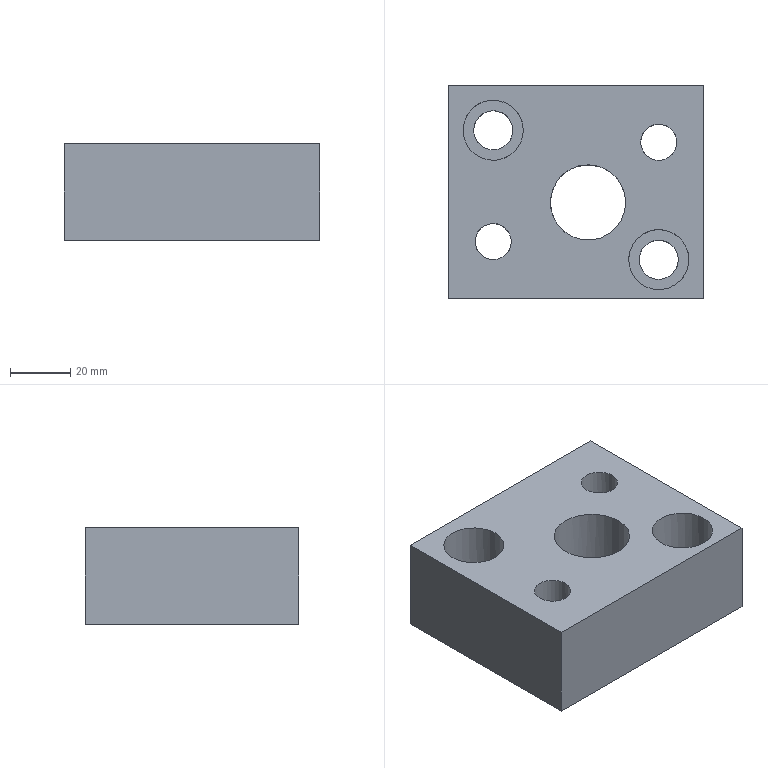Part | STEP file | gslz 2016.10.28-13_id1606_x_t | 1 solid | 17 faces | box 85 x 71 x 32 mm | volume 153487 mm3 | plane 9 | cylinder 8 | commonest cylinder face diameters 12 x2 13 x2 20 x2 25 x1 32 x1
STEP:
#1=CARTESIAN_POINT('',(0.,0.,0.));
#2=DIRECTION('',(0.,0.,1.));
#3=DIRECTION('',(1.,0.,0.));
#4=AXIS2_PLACEMENT_3D('',#1,#2,#3);
#5=CARTESIAN_POINT('',(-1393.372,235.,-32.));
#6=VERTEX_POINT('',#5);
#7=CARTESIAN_POINT('',(-1400.963,228.592,-32.));
#8=VERTEX_POINT('',#7);
#9=CARTESIAN_POINT('',(-1399.872,235.,-32.));
#10=DIRECTION('',(0.,0.,-1.));
#11=DIRECTION('',(1.,0.,0.));
#12=AXIS2_PLACEMENT_3D('',#9,#10,#11);
#13=CIRCLE('',#12,6.5);
#14=CARTESIAN_POINT('',(-1345.502,255.485,-32.));
#15=DIRECTION('',(0.,0.,1.));
#16=DIRECTION('',(1.,0.,0.));
#17=AXIS2_PLACEMENT_3D('',#14,#15,#16);
#18=PLANE('',#17);
#19=CARTESIAN_POINT('',(-47.871,-20.485));
#20=CARTESIAN_POINT('',(-47.871,-31.743));
#21=CARTESIAN_POINT('',(-57.621,-26.114));
#22=CARTESIAN_POINT('',(-67.371,-20.485));
#23=CARTESIAN_POINT('',(-57.621,-14.856));
#24=CARTESIAN_POINT('',(-47.871,-9.227));
#25=CARTESIAN_POINT('',(-47.871,-20.485));
#26=(BOUNDED_CURVE()B_SPLINE_CURVE(2,(#19,#20,#21,#22,#23,#24,#25),.UNSPECIFIED.,.T.,.F.)B_SPLINE_CURVE_WITH_KNOTS((1,2,2,2,2,1),(-2.094,0.,2.094,4.189,6.283,8.378),.UNSPECIFIED.)CURVE()GEOMETRIC_REPRESENTATION_ITEM()RATIONAL_B_SPLINE_CURVE((1.,0.5,1.,0.5,1.,0.5,1.))REPRESENTATION_ITEM(''));
#27=(GEOMETRIC_REPRESENTATION_CONTEXT(2)PARAMETRIC_REPRESENTATION_CONTEXT()REPRESENTATION_CONTEXT('',''));
#28=DEFINITIONAL_REPRESENTATION('',(#26),#27);
#29=PCURVE('',#18,#28);
#30=CARTESIAN_POINT('',(-1399.872,235.,-0.5408));
#31=DIRECTION('',(0.,0.,-1.));
#32=DIRECTION('',(-1.,0.,0.));
#33=AXIS2_PLACEMENT_3D('',#30,#31,#32);
#34=CYLINDRICAL_SURFACE('',#33,6.5);
#35=CARTESIAN_POINT('',(9.425,31.459));
#36=DIRECTION('',(1.,0.));
#37=VECTOR('',#36,1.);
#38=LINE('',#35,#37);
#39=(GEOMETRIC_REPRESENTATION_CONTEXT(2)PARAMETRIC_REPRESENTATION_CONTEXT()REPRESENTATION_CONTEXT('',''));
#40=DEFINITIONAL_REPRESENTATION('',(#38),#39);
#41=PCURVE('',#34,#40);
#42=SURFACE_CURVE('',#13,(#29,#41),.PCURVE_S1.);
#43=EDGE_CURVE('',#6,#8,#42,.T.);
#44=ORIENTED_EDGE('',*,*,#43,.F.);
#45=CARTESIAN_POINT('',(-1399.872,235.,-32.));
#46=DIRECTION('',(0.,0.,-1.));
#47=DIRECTION('',(1.,0.,0.));
#48=AXIS2_PLACEMENT_3D('',#45,#46,#47);
#49=CIRCLE('',#48,6.5);
#50=CARTESIAN_POINT('',(-47.871,-20.485));
#51=CARTESIAN_POINT('',(-47.871,-31.743));
#52=CARTESIAN_POINT('',(-57.621,-26.114));
#53=CARTESIAN_POINT('',(-67.371,-20.485));
#54=CARTESIAN_POINT('',(-57.621,-14.856));
#55=CARTESIAN_POINT('',(-47.871,-9.227));
#56=CARTESIAN_POINT('',(-47.871,-20.485));
#57=(BOUNDED_CURVE()B_SPLINE_CURVE(2,(#50,#51,#52,#53,#54,#55,#56),.UNSPECIFIED.,.T.,.F.)B_SPLINE_CURVE_WITH_KNOTS((1,2,2,2,2,1),(-2.094,0.,2.094,4.189,6.283,8.378),.UNSPECIFIED.)CURVE()GEOMETRIC_REPRESENTATION_ITEM()RATIONAL_B_SPLINE_CURVE((1.,0.5,1.,0.5,1.,0.5,1.))REPRESENTATION_ITEM(''));
#58=(GEOMETRIC_REPRESENTATION_CONTEXT(2)PARAMETRIC_REPRESENTATION_CONTEXT()REPRESENTATION_CONTEXT('',''));
#59=DEFINITIONAL_REPRESENTATION('',(#57),#58);
#60=PCURVE('',#18,#59);
#61=CARTESIAN_POINT('',(3.142,31.459));
#62=DIRECTION('',(1.,0.));
#63=VECTOR('',#62,1.);
#64=LINE('',#61,#63);
#65=(GEOMETRIC_REPRESENTATION_CONTEXT(2)PARAMETRIC_REPRESENTATION_CONTEXT()REPRESENTATION_CONTEXT('',''));
#66=DEFINITIONAL_REPRESENTATION('',(#64),#65);
#67=PCURVE('',#34,#66);
#68=SURFACE_CURVE('',#49,(#60,#67),.PCURVE_S1.);
#69=EDGE_CURVE('',#8,#6,#68,.T.);
#70=ORIENTED_EDGE('',*,*,#69,.F.);
#71=EDGE_LOOP('',(#44,#70));
#72=FACE_BOUND('',#71,.T.);
#73=CARTESIAN_POINT('',(-1453.551,246.853,-32.));
#74=VERTEX_POINT('',#73);
#75=CARTESIAN_POINT('',(-1454.872,241.,-32.));
#76=DIRECTION('',(0.,0.,1.));
#77=DIRECTION('',(0.2202,0.9754,0.));
#78=AXIS2_PLACEMENT_3D('',#75,#76,#77);
#79=CIRCLE('',#78,6.);
#80=CARTESIAN_POINT('',(-109.371,-14.485));
#81=DIRECTION('',(0.2202,0.9754));
#82=AXIS2_PLACEMENT_2D('',#80,#81);
#83=CIRCLE('',#82,6.);
#84=(GEOMETRIC_REPRESENTATION_CONTEXT(2)PARAMETRIC_REPRESENTATION_CONTEXT()REPRESENTATION_CONTEXT('',''));
#85=DEFINITIONAL_REPRESENTATION('',(#83),#84);
#86=PCURVE('',#18,#85);
#87=CARTESIAN_POINT('',(-1454.872,241.,-9.));
#88=DIRECTION('',(0.,0.,-1.));
#89=DIRECTION('',(-1.,0.,0.));
#90=AXIS2_PLACEMENT_3D('',#87,#88,#89);
#91=CYLINDRICAL_SURFACE('',#90,6.);
#92=CARTESIAN_POINT('',(8.076,23.));
#93=DIRECTION('',(-1.,0.));
#94=VECTOR('',#93,1.);
#95=LINE('',#92,#94);
#96=(GEOMETRIC_REPRESENTATION_CONTEXT(2)PARAMETRIC_REPRESENTATION_CONTEXT()REPRESENTATION_CONTEXT('',''));
#97=DEFINITIONAL_REPRESENTATION('',(#95),#96);
#98=PCURVE('',#91,#97);
#99=SURFACE_CURVE('',#79,(#86,#98),.PCURVE_S1.);
#100=EDGE_CURVE('',#74,#74,#99,.T.);
#101=ORIENTED_EDGE('',*,*,#100,.T.);
#102=EDGE_LOOP('',(#101));
#103=FACE_BOUND('',#102,.T.);
#104=CARTESIAN_POINT('',(-1448.372,278.,-32.));
#105=VERTEX_POINT('',#104);
#106=CARTESIAN_POINT('',(-1455.963,271.592,-32.));
#107=VERTEX_POINT('',#106);
#108=CARTESIAN_POINT('',(-1454.872,278.,-32.));
#109=DIRECTION('',(0.,0.,-1.));
#110=DIRECTION('',(1.,0.,0.));
#111=AXIS2_PLACEMENT_3D('',#108,#109,#110);
#112=CIRCLE('',#111,6.5);
#113=CARTESIAN_POINT('',(-102.871,22.515));
#114=CARTESIAN_POINT('',(-102.871,11.257));
#115=CARTESIAN_POINT('',(-112.621,16.886));
#116=CARTESIAN_POINT('',(-122.371,22.515));
#117=CARTESIAN_POINT('',(-112.621,28.144));
#118=CARTESIAN_POINT('',(-102.871,33.773));
#119=CARTESIAN_POINT('',(-102.871,22.515));
#120=(BOUNDED_CURVE()B_SPLINE_CURVE(2,(#113,#114,#115,#116,#117,#118,#119),.UNSPECIFIED.,.T.,.F.)B_SPLINE_CURVE_WITH_KNOTS((1,2,2,2,2,1),(-2.094,0.,2.094,4.189,6.283,8.378),.UNSPECIFIED.)CURVE()GEOMETRIC_REPRESENTATION_ITEM()RATIONAL_B_SPLINE_CURVE((1.,0.5,1.,0.5,1.,0.5,1.))REPRESENTATION_ITEM(''));
#121=(GEOMETRIC_REPRESENTATION_CONTEXT(2)PARAMETRIC_REPRESENTATION_CONTEXT()REPRESENTATION_CONTEXT('',''));
#122=DEFINITIONAL_REPRESENTATION('',(#120),#121);
#123=PCURVE('',#18,#122);
#124=CARTESIAN_POINT('',(-1454.872,278.,-0.5408));
#125=DIRECTION('',(0.,0.,-1.));
#126=DIRECTION('',(-1.,0.,0.));
#127=AXIS2_PLACEMENT_3D('',#124,#125,#126);
#128=CYLINDRICAL_SURFACE('',#127,6.5);
#129=CARTESIAN_POINT('',(9.425,31.459));
#130=DIRECTION('',(1.,0.));
#131=VECTOR('',#130,1.);
#132=LINE('',#129,#131);
#133=(GEOMETRIC_REPRESENTATION_CONTEXT(2)PARAMETRIC_REPRESENTATION_CONTEXT()REPRESENTATION_CONTEXT('',''));
#134=DEFINITIONAL_REPRESENTATION('',(#132),#133);
#135=PCURVE('',#128,#134);
#136=SURFACE_CURVE('',#112,(#123,#135),.PCURVE_S1.);
#137=EDGE_CURVE('',#105,#107,#136,.T.);
#138=ORIENTED_EDGE('',*,*,#137,.F.);
#139=CARTESIAN_POINT('',(-1454.872,278.,-32.));
#140=DIRECTION('',(0.,0.,-1.));
#141=DIRECTION('',(1.,0.,0.));
#142=AXIS2_PLACEMENT_3D('',#139,#140,#141);
#143=CIRCLE('',#142,6.5);
#144=CARTESIAN_POINT('',(-102.871,22.515));
#145=CARTESIAN_POINT('',(-102.871,11.257));
#146=CARTESIAN_POINT('',(-112.621,16.886));
#147=CARTESIAN_POINT('',(-122.371,22.515));
#148=CARTESIAN_POINT('',(-112.621,28.144));
#149=CARTESIAN_POINT('',(-102.871,33.773));
#150=CARTESIAN_POINT('',(-102.871,22.515));
#151=(BOUNDED_CURVE()B_SPLINE_CURVE(2,(#144,#145,#146,#147,#148,#149,#150),.UNSPECIFIED.,.T.,.F.)B_SPLINE_CURVE_WITH_KNOTS((1,2,2,2,2,1),(-2.094,0.,2.094,4.189,6.283,8.378),.UNSPECIFIED.)CURVE()GEOMETRIC_REPRESENTATION_ITEM()RATIONAL_B_SPLINE_CURVE((1.,0.5,1.,0.5,1.,0.5,1.))REPRESENTATION_ITEM(''));
#152=(GEOMETRIC_REPRESENTATION_CONTEXT(2)PARAMETRIC_REPRESENTATION_CONTEXT()REPRESENTATION_CONTEXT('',''));
#153=DEFINITIONAL_REPRESENTATION('',(#151),#152);
#154=PCURVE('',#18,#153);
#155=CARTESIAN_POINT('',(3.142,31.459));
#156=DIRECTION('',(1.,0.));
#157=VECTOR('',#156,1.);
#158=LINE('',#155,#157);
#159=(GEOMETRIC_REPRESENTATION_CONTEXT(2)PARAMETRIC_REPRESENTATION_CONTEXT()REPRESENTATION_CONTEXT('',''));
#160=DEFINITIONAL_REPRESENTATION('',(#158),#159);
#161=PCURVE('',#128,#160);
#162=SURFACE_CURVE('',#143,(#154,#161),.PCURVE_S1.);
#163=EDGE_CURVE('',#107,#105,#162,.T.);
#164=ORIENTED_EDGE('',*,*,#163,.F.);
#165=EDGE_LOOP('',(#138,#164));
#166=FACE_BOUND('',#165,.T.);
#167=CARTESIAN_POINT('',(-1384.872,293.,-32.));
#168=VERTEX_POINT('',#167);
#169=CARTESIAN_POINT('',(-1469.872,293.,-32.));
#170=VERTEX_POINT('',#169);
#171=CARTESIAN_POINT('',(-1423.372,293.,-32.));
#172=DIRECTION('',(-1.,0.,0.));
#173=VECTOR('',#172,1.);
#174=LINE('',#171,#173);
#175=CARTESIAN_POINT('',(-77.871,37.515));
#176=DIRECTION('',(-1.,0.));
#177=VECTOR('',#176,1.);
#178=LINE('',#175,#177);
#179=(GEOMETRIC_REPRESENTATION_CONTEXT(2)PARAMETRIC_REPRESENTATION_CONTEXT()REPRESENTATION_CONTEXT('',''));
#180=DEFINITIONAL_REPRESENTATION('',(#178),#179);
#181=PCURVE('',#18,#180);
#182=CARTESIAN_POINT('',(-1423.372,293.,-56.));
#183=DIRECTION('',(0.,1.,0.));
#184=DIRECTION('',(0.,0.,1.));
#185=AXIS2_PLACEMENT_3D('',#182,#183,#184);
#186=PLANE('',#185);
#187=CARTESIAN_POINT('',(24.,0.));
#188=DIRECTION('',(0.,-1.));
#189=VECTOR('',#188,1.);
#190=LINE('',#187,#189);
#191=(GEOMETRIC_REPRESENTATION_CONTEXT(2)PARAMETRIC_REPRESENTATION_CONTEXT()REPRESENTATION_CONTEXT('',''));
#192=DEFINITIONAL_REPRESENTATION('',(#190),#191);
#193=PCURVE('',#186,#192);
#194=SURFACE_CURVE('',#174,(#181,#193),.PCURVE_S1.);
#195=EDGE_CURVE('',#168,#170,#194,.T.);
#196=ORIENTED_EDGE('',*,*,#195,.F.);
#197=CARTESIAN_POINT('',(-1384.872,222.,-32.));
#198=VERTEX_POINT('',#197);
#199=CARTESIAN_POINT('',(-1384.872,336.,-32.));
#200=DIRECTION('',(0.,1.,0.));
#201=VECTOR('',#200,1.);
#202=LINE('',#199,#201);
#203=CARTESIAN_POINT('',(-39.371,80.515));
#204=DIRECTION('',(0.,1.));
#205=VECTOR('',#204,1.);
#206=LINE('',#203,#205);
#207=(GEOMETRIC_REPRESENTATION_CONTEXT(2)PARAMETRIC_REPRESENTATION_CONTEXT()REPRESENTATION_CONTEXT('',''));
#208=DEFINITIONAL_REPRESENTATION('',(#206),#207);
#209=PCURVE('',#18,#208);
#210=CARTESIAN_POINT('',(-1384.872,336.,-56.));
#211=DIRECTION('',(1.,0.,0.));
#212=DIRECTION('',(0.,0.,-1.));
#213=AXIS2_PLACEMENT_3D('',#210,#211,#212);
#214=PLANE('',#213);
#215=CARTESIAN_POINT('',(-24.,0.));
#216=DIRECTION('',(0.,1.));
#217=VECTOR('',#216,1.);
#218=LINE('',#215,#217);
#219=(GEOMETRIC_REPRESENTATION_CONTEXT(2)PARAMETRIC_REPRESENTATION_CONTEXT()REPRESENTATION_CONTEXT('',''));
#220=DEFINITIONAL_REPRESENTATION('',(#218),#219);
#221=PCURVE('',#214,#220);
#222=SURFACE_CURVE('',#202,(#209,#221),.PCURVE_S1.);
#223=EDGE_CURVE('',#198,#168,#222,.T.);
#224=ORIENTED_EDGE('',*,*,#223,.F.);
#225=CARTESIAN_POINT('',(-1469.872,222.,-32.));
#226=VERTEX_POINT('',#225);
#227=CARTESIAN_POINT('',(-1423.372,222.,-32.));
#228=DIRECTION('',(1.,0.,0.));
#229=VECTOR('',#228,1.);
#230=LINE('',#227,#229);
#231=CARTESIAN_POINT('',(-77.871,-33.485));
#232=DIRECTION('',(1.,0.));
#233=VECTOR('',#232,1.);
#234=LINE('',#231,#233);
#235=(GEOMETRIC_REPRESENTATION_CONTEXT(2)PARAMETRIC_REPRESENTATION_CONTEXT()REPRESENTATION_CONTEXT('',''));
#236=DEFINITIONAL_REPRESENTATION('',(#234),#235);
#237=PCURVE('',#18,#236);
#238=CARTESIAN_POINT('',(-1423.372,222.,-56.));
#239=DIRECTION('',(0.,-1.,0.));
#240=DIRECTION('',(0.,0.,-1.));
#241=AXIS2_PLACEMENT_3D('',#238,#239,#240);
#242=PLANE('',#241);
#243=CARTESIAN_POINT('',(-24.,0.));
#244=DIRECTION('',(0.,1.));
#245=VECTOR('',#244,1.);
#246=LINE('',#243,#245);
#247=(GEOMETRIC_REPRESENTATION_CONTEXT(2)PARAMETRIC_REPRESENTATION_CONTEXT()REPRESENTATION_CONTEXT('',''));
#248=DEFINITIONAL_REPRESENTATION('',(#246),#247);
#249=PCURVE('',#242,#248);
#250=SURFACE_CURVE('',#230,(#237,#249),.PCURVE_S1.);
#251=EDGE_CURVE('',#226,#198,#250,.T.);
#252=ORIENTED_EDGE('',*,*,#251,.F.);
#253=CARTESIAN_POINT('',(-1469.872,336.,-32.));
#254=DIRECTION('',(0.,-1.,0.));
#255=VECTOR('',#254,1.);
#256=LINE('',#253,#255);
#257=CARTESIAN_POINT('',(-124.371,80.515));
#258=DIRECTION('',(0.,-1.));
#259=VECTOR('',#258,1.);
#260=LINE('',#257,#259);
#261=(GEOMETRIC_REPRESENTATION_CONTEXT(2)PARAMETRIC_REPRESENTATION_CONTEXT()REPRESENTATION_CONTEXT('',''));
#262=DEFINITIONAL_REPRESENTATION('',(#260),#261);
#263=PCURVE('',#18,#262);
#264=CARTESIAN_POINT('',(-1469.872,336.,-56.));
#265=DIRECTION('',(-1.,0.,0.));
#266=DIRECTION('',(0.,0.,1.));
#267=AXIS2_PLACEMENT_3D('',#264,#265,#266);
#268=PLANE('',#267);
#269=CARTESIAN_POINT('',(24.,0.));
#270=DIRECTION('',(0.,-1.));
#271=VECTOR('',#270,1.);
#272=LINE('',#269,#271);
#273=(GEOMETRIC_REPRESENTATION_CONTEXT(2)PARAMETRIC_REPRESENTATION_CONTEXT()REPRESENTATION_CONTEXT('',''));
#274=DEFINITIONAL_REPRESENTATION('',(#272),#273);
#275=PCURVE('',#268,#274);
#276=SURFACE_CURVE('',#256,(#263,#275),.PCURVE_S1.);
#277=EDGE_CURVE('',#170,#226,#276,.T.);
#278=ORIENTED_EDGE('',*,*,#277,.F.);
#279=EDGE_LOOP('',(#196,#224,#252,#278));
#280=FACE_BOUND('',#279,.T.);
#281=CARTESIAN_POINT('',(-1407.372,254.,-32.));
#282=VERTEX_POINT('',#281);
#283=CARTESIAN_POINT('',(-1423.372,254.,-32.));
#284=DIRECTION('',(0.,0.,-1.));
#285=DIRECTION('',(1.,0.,0.));
#286=AXIS2_PLACEMENT_3D('',#283,#284,#285);
#287=CIRCLE('',#286,16.);
#288=CARTESIAN_POINT('',(-61.871,-1.485));
#289=CARTESIAN_POINT('',(-61.871,-29.198));
#290=CARTESIAN_POINT('',(-85.871,-15.341));
#291=CARTESIAN_POINT('',(-109.871,-1.485));
#292=CARTESIAN_POINT('',(-85.871,12.372));
#293=CARTESIAN_POINT('',(-61.871,26.228));
#294=CARTESIAN_POINT('',(-61.871,-1.485));
#295=(BOUNDED_CURVE()B_SPLINE_CURVE(2,(#288,#289,#290,#291,#292,#293,#294),.UNSPECIFIED.,.T.,.F.)B_SPLINE_CURVE_WITH_KNOTS((1,2,2,2,2,1),(-2.094,0.,2.094,4.189,6.283,8.378),.UNSPECIFIED.)CURVE()GEOMETRIC_REPRESENTATION_ITEM()RATIONAL_B_SPLINE_CURVE((1.,0.5,1.,0.5,1.,0.5,1.))REPRESENTATION_ITEM(''));
#296=(GEOMETRIC_REPRESENTATION_CONTEXT(2)PARAMETRIC_REPRESENTATION_CONTEXT()REPRESENTATION_CONTEXT('',''));
#297=DEFINITIONAL_REPRESENTATION('',(#295),#296);
#298=PCURVE('',#18,#297);
#299=CARTESIAN_POINT('',(-1423.372,254.,-32.5));
#300=DIRECTION('',(0.,0.,1.));
#301=DIRECTION('',(0.,-1.,0.));
#302=AXIS2_PLACEMENT_3D('',#299,#300,#301);
#303=CYLINDRICAL_SURFACE('',#302,16.);
#304=CARTESIAN_POINT('',(7.854,0.5));
#305=DIRECTION('',(-1.,0.));
#306=VECTOR('',#305,1.);
#307=LINE('',#304,#306);
#308=(GEOMETRIC_REPRESENTATION_CONTEXT(2)PARAMETRIC_REPRESENTATION_CONTEXT()REPRESENTATION_CONTEXT('',''));
#309=DEFINITIONAL_REPRESENTATION('',(#307),#308);
#310=PCURVE('',#303,#309);
#311=SURFACE_CURVE('',#287,(#298,#310),.PCURVE_S1.);
#312=EDGE_CURVE('',#282,#282,#311,.T.);
#313=ORIENTED_EDGE('',*,*,#312,.F.);
#314=EDGE_LOOP('',(#313));
#315=FACE_BOUND('',#314,.T.);
#316=CARTESIAN_POINT('',(-1398.551,279.853,-32.));
#317=VERTEX_POINT('',#316);
#318=CARTESIAN_POINT('',(-1399.872,274.,-32.));
#319=DIRECTION('',(0.,0.,1.));
#320=DIRECTION('',(0.2202,0.9754,0.));
#321=AXIS2_PLACEMENT_3D('',#318,#319,#320);
#322=CIRCLE('',#321,6.);
#323=CARTESIAN_POINT('',(-54.371,18.515));
#324=DIRECTION('',(0.2202,0.9754));
#325=AXIS2_PLACEMENT_2D('',#323,#324);
#326=CIRCLE('',#325,6.);
#327=(GEOMETRIC_REPRESENTATION_CONTEXT(2)PARAMETRIC_REPRESENTATION_CONTEXT()REPRESENTATION_CONTEXT('',''));
#328=DEFINITIONAL_REPRESENTATION('',(#326),#327);
#329=PCURVE('',#18,#328);
#330=CARTESIAN_POINT('',(-1399.872,274.,-9.));
#331=DIRECTION('',(0.,0.,-1.));
#332=DIRECTION('',(-1.,0.,0.));
#333=AXIS2_PLACEMENT_3D('',#330,#331,#332);
#334=CYLINDRICAL_SURFACE('',#333,6.);
#335=CARTESIAN_POINT('',(8.076,23.));
#336=DIRECTION('',(-1.,0.));
#337=VECTOR('',#336,1.);
#338=LINE('',#335,#337);
#339=(GEOMETRIC_REPRESENTATION_CONTEXT(2)PARAMETRIC_REPRESENTATION_CONTEXT()REPRESENTATION_CONTEXT('',''));
#340=DEFINITIONAL_REPRESENTATION('',(#338),#339);
#341=PCURVE('',#334,#340);
#342=SURFACE_CURVE('',#322,(#329,#341),.PCURVE_S1.);
#343=EDGE_CURVE('',#317,#317,#342,.T.);
#344=ORIENTED_EDGE('',*,*,#343,.T.);
#345=EDGE_LOOP('',(#344));
#346=FACE_BOUND('',#345,.T.);
#347=ADVANCED_FACE('',(#72,#103,#166,#280,#315,#346),#18,.F.);
#348=CARTESIAN_POINT('',(-1389.872,235.,0.));
#349=VERTEX_POINT('',#348);
#350=CARTESIAN_POINT('',(-1401.551,225.142,0.));
#351=VERTEX_POINT('',#350);
#352=CARTESIAN_POINT('',(-1399.872,235.,0.));
#353=DIRECTION('',(0.,0.,1.));
#354=DIRECTION('',(1.,0.,0.));
#355=AXIS2_PLACEMENT_3D('',#352,#353,#354);
#356=CIRCLE('',#355,10.);
#357=CARTESIAN_POINT('',(-1423.372,336.,0.));
#358=DIRECTION('',(0.,0.,1.));
#359=DIRECTION('',(0.,-1.,0.));
#360=AXIS2_PLACEMENT_3D('',#357,#358,#359);
#361=PLANE('',#360);
#362=CARTESIAN_POINT('',(101.,23.5));
#363=DIRECTION('',(0.,1.));
#364=AXIS2_PLACEMENT_2D('',#362,#363);
#365=CIRCLE('',#364,10.);
#366=(GEOMETRIC_REPRESENTATION_CONTEXT(2)PARAMETRIC_REPRESENTATION_CONTEXT()REPRESENTATION_CONTEXT('',''));
#367=DEFINITIONAL_REPRESENTATION('',(#365),#366);
#368=PCURVE('',#361,#367);
#369=CARTESIAN_POINT('',(-1399.872,235.,-0.5408));
#370=DIRECTION('',(0.,0.,-1.));
#371=DIRECTION('',(-1.,0.,0.));
#372=AXIS2_PLACEMENT_3D('',#369,#370,#371);
#373=CYLINDRICAL_SURFACE('',#372,10.);
#374=CARTESIAN_POINT('',(9.425,-0.5408));
#375=DIRECTION('',(-1.,0.));
#376=VECTOR('',#375,1.);
#377=LINE('',#374,#376);
#378=(GEOMETRIC_REPRESENTATION_CONTEXT(2)PARAMETRIC_REPRESENTATION_CONTEXT()REPRESENTATION_CONTEXT('',''));
#379=DEFINITIONAL_REPRESENTATION('',(#377),#378);
#380=PCURVE('',#373,#379);
#381=SURFACE_CURVE('',#356,(#368,#380),.PCURVE_S1.);
#382=EDGE_CURVE('',#349,#351,#381,.T.);
#383=ORIENTED_EDGE('',*,*,#382,.F.);
#384=CARTESIAN_POINT('',(-1399.872,235.,0.));
#385=DIRECTION('',(0.,0.,1.));
#386=DIRECTION('',(1.,0.,0.));
#387=AXIS2_PLACEMENT_3D('',#384,#385,#386);
#388=CIRCLE('',#387,10.);
#389=CARTESIAN_POINT('',(101.,23.5));
#390=DIRECTION('',(0.,1.));
#391=AXIS2_PLACEMENT_2D('',#389,#390);
#392=CIRCLE('',#391,10.);
#393=(GEOMETRIC_REPRESENTATION_CONTEXT(2)PARAMETRIC_REPRESENTATION_CONTEXT()REPRESENTATION_CONTEXT('',''));
#394=DEFINITIONAL_REPRESENTATION('',(#392),#393);
#395=PCURVE('',#361,#394);
#396=CARTESIAN_POINT('',(15.708,-0.5408));
#397=DIRECTION('',(-1.,0.));
#398=VECTOR('',#397,1.);
#399=LINE('',#396,#398);
#400=(GEOMETRIC_REPRESENTATION_CONTEXT(2)PARAMETRIC_REPRESENTATION_CONTEXT()REPRESENTATION_CONTEXT('',''));
#401=DEFINITIONAL_REPRESENTATION('',(#399),#400);
#402=PCURVE('',#373,#401);
#403=SURFACE_CURVE('',#388,(#395,#402),.PCURVE_S1.);
#404=EDGE_CURVE('',#351,#349,#403,.T.);
#405=ORIENTED_EDGE('',*,*,#404,.F.);
#406=EDGE_LOOP('',(#383,#405));
#407=FACE_BOUND('',#406,.T.);
#408=CARTESIAN_POINT('',(-1393.872,274.,0.));
#409=VERTEX_POINT('',#408);
#410=CARTESIAN_POINT('',(-1398.551,279.853,0.));
#411=VERTEX_POINT('',#410);
#412=CARTESIAN_POINT('',(-1399.872,274.,0.));
#413=DIRECTION('',(0.,0.,1.));
#414=DIRECTION('',(1.,0.,0.));
#415=AXIS2_PLACEMENT_3D('',#412,#413,#414);
#416=CIRCLE('',#415,6.);
#417=CARTESIAN_POINT('',(62.,23.5));
#418=DIRECTION('',(0.,1.));
#419=AXIS2_PLACEMENT_2D('',#417,#418);
#420=CIRCLE('',#419,6.);
#421=(GEOMETRIC_REPRESENTATION_CONTEXT(2)PARAMETRIC_REPRESENTATION_CONTEXT()REPRESENTATION_CONTEXT('',''));
#422=DEFINITIONAL_REPRESENTATION('',(#420),#421);
#423=PCURVE('',#361,#422);
#424=CARTESIAN_POINT('',(3.142,-9.));
#425=DIRECTION('',(-1.,0.));
#426=VECTOR('',#425,1.);
#427=LINE('',#424,#426);
#428=(GEOMETRIC_REPRESENTATION_CONTEXT(2)PARAMETRIC_REPRESENTATION_CONTEXT()REPRESENTATION_CONTEXT('',''));
#429=DEFINITIONAL_REPRESENTATION('',(#427),#428);
#430=PCURVE('',#334,#429);
#431=SURFACE_CURVE('',#416,(#423,#430),.PCURVE_S1.);
#432=EDGE_CURVE('',#409,#411,#431,.T.);
#433=ORIENTED_EDGE('',*,*,#432,.F.);
#434=CARTESIAN_POINT('',(-1399.872,274.,0.));
#435=DIRECTION('',(0.,0.,1.));
#436=DIRECTION('',(1.,0.,0.));
#437=AXIS2_PLACEMENT_3D('',#434,#435,#436);
#438=CIRCLE('',#437,6.);
#439=CARTESIAN_POINT('',(62.,23.5));
#440=DIRECTION('',(0.,1.));
#441=AXIS2_PLACEMENT_2D('',#439,#440);
#442=CIRCLE('',#441,6.);
#443=(GEOMETRIC_REPRESENTATION_CONTEXT(2)PARAMETRIC_REPRESENTATION_CONTEXT()REPRESENTATION_CONTEXT('',''));
#444=DEFINITIONAL_REPRESENTATION('',(#442),#443);
#445=PCURVE('',#361,#444);
#446=CARTESIAN_POINT('',(9.425,-9.));
#447=DIRECTION('',(-1.,0.));
#448=VECTOR('',#447,1.);
#449=LINE('',#446,#448);
#450=(GEOMETRIC_REPRESENTATION_CONTEXT(2)PARAMETRIC_REPRESENTATION_CONTEXT()REPRESENTATION_CONTEXT('',''));
#451=DEFINITIONAL_REPRESENTATION('',(#449),#450);
#452=PCURVE('',#334,#451);
#453=SURFACE_CURVE('',#438,(#445,#452),.PCURVE_S1.);
#454=EDGE_CURVE('',#411,#409,#453,.T.);
#455=ORIENTED_EDGE('',*,*,#454,.F.);
#456=EDGE_LOOP('',(#433,#455));
#457=FACE_BOUND('',#456,.T.);
#458=CARTESIAN_POINT('',(-1448.872,241.,0.));
#459=VERTEX_POINT('',#458);
#460=CARTESIAN_POINT('',(-1453.551,246.853,0.));
#461=VERTEX_POINT('',#460);
#462=CARTESIAN_POINT('',(-1454.872,241.,0.));
#463=DIRECTION('',(0.,0.,1.));
#464=DIRECTION('',(1.,0.,0.));
#465=AXIS2_PLACEMENT_3D('',#462,#463,#464);
#466=CIRCLE('',#465,6.);
#467=CARTESIAN_POINT('',(95.,-31.5));
#468=DIRECTION('',(0.,1.));
#469=AXIS2_PLACEMENT_2D('',#467,#468);
#470=CIRCLE('',#469,6.);
#471=(GEOMETRIC_REPRESENTATION_CONTEXT(2)PARAMETRIC_REPRESENTATION_CONTEXT()REPRESENTATION_CONTEXT('',''));
#472=DEFINITIONAL_REPRESENTATION('',(#470),#471);
#473=PCURVE('',#361,#472);
#474=CARTESIAN_POINT('',(3.142,-9.));
#475=DIRECTION('',(-1.,0.));
#476=VECTOR('',#475,1.);
#477=LINE('',#474,#476);
#478=(GEOMETRIC_REPRESENTATION_CONTEXT(2)PARAMETRIC_REPRESENTATION_CONTEXT()REPRESENTATION_CONTEXT('',''));
#479=DEFINITIONAL_REPRESENTATION('',(#477),#478);
#480=PCURVE('',#91,#479);
#481=SURFACE_CURVE('',#466,(#473,#480),.PCURVE_S1.);
#482=EDGE_CURVE('',#459,#461,#481,.T.);
#483=ORIENTED_EDGE('',*,*,#482,.F.);
#484=CARTESIAN_POINT('',(-1454.872,241.,0.));
#485=DIRECTION('',(0.,0.,1.));
#486=DIRECTION('',(1.,0.,0.));
#487=AXIS2_PLACEMENT_3D('',#484,#485,#486);
#488=CIRCLE('',#487,6.);
#489=CARTESIAN_POINT('',(95.,-31.5));
#490=DIRECTION('',(0.,1.));
#491=AXIS2_PLACEMENT_2D('',#489,#490);
#492=CIRCLE('',#491,6.);
#493=(GEOMETRIC_REPRESENTATION_CONTEXT(2)PARAMETRIC_REPRESENTATION_CONTEXT()REPRESENTATION_CONTEXT('',''));
#494=DEFINITIONAL_REPRESENTATION('',(#492),#493);
#495=PCURVE('',#361,#494);
#496=CARTESIAN_POINT('',(9.425,-9.));
#497=DIRECTION('',(-1.,0.));
#498=VECTOR('',#497,1.);
#499=LINE('',#496,#498);
#500=(GEOMETRIC_REPRESENTATION_CONTEXT(2)PARAMETRIC_REPRESENTATION_CONTEXT()REPRESENTATION_CONTEXT('',''));
#501=DEFINITIONAL_REPRESENTATION('',(#499),#500);
#502=PCURVE('',#91,#501);
#503=SURFACE_CURVE('',#488,(#495,#502),.PCURVE_S1.);
#504=EDGE_CURVE('',#461,#459,#503,.T.);
#505=ORIENTED_EDGE('',*,*,#504,.F.);
#506=EDGE_LOOP('',(#483,#505));
#507=FACE_BOUND('',#506,.T.);
#508=CARTESIAN_POINT('',(-1444.872,278.,0.));
#509=VERTEX_POINT('',#508);
#510=CARTESIAN_POINT('',(-1456.551,268.142,0.));
#511=VERTEX_POINT('',#510);
#512=CARTESIAN_POINT('',(-1454.872,278.,0.));
#513=DIRECTION('',(0.,0.,1.));
#514=DIRECTION('',(1.,0.,0.));
#515=AXIS2_PLACEMENT_3D('',#512,#513,#514);
#516=CIRCLE('',#515,10.);
#517=CARTESIAN_POINT('',(58.,-31.5));
#518=DIRECTION('',(0.,1.));
#519=AXIS2_PLACEMENT_2D('',#517,#518);
#520=CIRCLE('',#519,10.);
#521=(GEOMETRIC_REPRESENTATION_CONTEXT(2)PARAMETRIC_REPRESENTATION_CONTEXT()REPRESENTATION_CONTEXT('',''));
#522=DEFINITIONAL_REPRESENTATION('',(#520),#521);
#523=PCURVE('',#361,#522);
#524=CARTESIAN_POINT('',(-1454.872,278.,-0.5408));
#525=DIRECTION('',(0.,0.,-1.));
#526=DIRECTION('',(-1.,0.,0.));
#527=AXIS2_PLACEMENT_3D('',#524,#525,#526);
#528=CYLINDRICAL_SURFACE('',#527,10.);
#529=CARTESIAN_POINT('',(9.425,-0.5408));
#530=DIRECTION('',(-1.,0.));
#531=VECTOR('',#530,1.);
#532=LINE('',#529,#531);
#533=(GEOMETRIC_REPRESENTATION_CONTEXT(2)PARAMETRIC_REPRESENTATION_CONTEXT()REPRESENTATION_CONTEXT('',''));
#534=DEFINITIONAL_REPRESENTATION('',(#532),#533);
#535=PCURVE('',#528,#534);
#536=SURFACE_CURVE('',#516,(#523,#535),.PCURVE_S1.);
#537=EDGE_CURVE('',#509,#511,#536,.T.);
#538=ORIENTED_EDGE('',*,*,#537,.F.);
#539=CARTESIAN_POINT('',(-1454.872,278.,0.));
#540=DIRECTION('',(0.,0.,1.));
#541=DIRECTION('',(1.,0.,0.));
#542=AXIS2_PLACEMENT_3D('',#539,#540,#541);
#543=CIRCLE('',#542,10.);
#544=CARTESIAN_POINT('',(58.,-31.5));
#545=DIRECTION('',(0.,1.));
#546=AXIS2_PLACEMENT_2D('',#544,#545);
#547=CIRCLE('',#546,10.);
#548=(GEOMETRIC_REPRESENTATION_CONTEXT(2)PARAMETRIC_REPRESENTATION_CONTEXT()REPRESENTATION_CONTEXT('',''));
#549=DEFINITIONAL_REPRESENTATION('',(#547),#548);
#550=PCURVE('',#361,#549);
#551=CARTESIAN_POINT('',(15.708,-0.5408));
#552=DIRECTION('',(-1.,0.));
#553=VECTOR('',#552,1.);
#554=LINE('',#551,#553);
#555=(GEOMETRIC_REPRESENTATION_CONTEXT(2)PARAMETRIC_REPRESENTATION_CONTEXT()REPRESENTATION_CONTEXT('',''));
#556=DEFINITIONAL_REPRESENTATION('',(#554),#555);
#557=PCURVE('',#528,#556);
#558=SURFACE_CURVE('',#543,(#550,#557),.PCURVE_S1.);
#559=EDGE_CURVE('',#511,#509,#558,.T.);
#560=ORIENTED_EDGE('',*,*,#559,.F.);
#561=EDGE_LOOP('',(#538,#560));
#562=FACE_BOUND('',#561,.T.);
#563=CARTESIAN_POINT('',(-1384.872,293.,0.));
#564=VERTEX_POINT('',#563);
#565=CARTESIAN_POINT('',(-1384.872,222.,0.));
#566=VERTEX_POINT('',#565);
#567=CARTESIAN_POINT('',(-1384.872,336.,0.));
#568=DIRECTION('',(0.,-1.,0.));
#569=VECTOR('',#568,1.);
#570=LINE('',#567,#569);
#571=CARTESIAN_POINT('',(0.,38.5));
#572=DIRECTION('',(1.,0.));
#573=VECTOR('',#572,1.);
#574=LINE('',#571,#573);
#575=(GEOMETRIC_REPRESENTATION_CONTEXT(2)PARAMETRIC_REPRESENTATION_CONTEXT()REPRESENTATION_CONTEXT('',''));
#576=DEFINITIONAL_REPRESENTATION('',(#574),#575);
#577=PCURVE('',#361,#576);
#578=CARTESIAN_POINT('',(-56.,0.));
#579=DIRECTION('',(0.,-1.));
#580=VECTOR('',#579,1.);
#581=LINE('',#578,#580);
#582=(GEOMETRIC_REPRESENTATION_CONTEXT(2)PARAMETRIC_REPRESENTATION_CONTEXT()REPRESENTATION_CONTEXT('',''));
#583=DEFINITIONAL_REPRESENTATION('',(#581),#582);
#584=PCURVE('',#214,#583);
#585=SURFACE_CURVE('',#570,(#577,#584),.PCURVE_S1.);
#586=EDGE_CURVE('',#564,#566,#585,.T.);
#587=ORIENTED_EDGE('',*,*,#586,.F.);
#588=CARTESIAN_POINT('',(-1469.872,293.,0.));
#589=VERTEX_POINT('',#588);
#590=CARTESIAN_POINT('',(-1423.372,293.,0.));
#591=DIRECTION('',(1.,0.,0.));
#592=VECTOR('',#591,1.);
#593=LINE('',#590,#592);
#594=CARTESIAN_POINT('',(43.,0.));
#595=DIRECTION('',(0.,1.));
#596=VECTOR('',#595,1.);
#597=LINE('',#594,#596);
#598=(GEOMETRIC_REPRESENTATION_CONTEXT(2)PARAMETRIC_REPRESENTATION_CONTEXT()REPRESENTATION_CONTEXT('',''));
#599=DEFINITIONAL_REPRESENTATION('',(#597),#598);
#600=PCURVE('',#361,#599);
#601=CARTESIAN_POINT('',(56.,0.));
#602=DIRECTION('',(0.,1.));
#603=VECTOR('',#602,1.);
#604=LINE('',#601,#603);
#605=(GEOMETRIC_REPRESENTATION_CONTEXT(2)PARAMETRIC_REPRESENTATION_CONTEXT()REPRESENTATION_CONTEXT('',''));
#606=DEFINITIONAL_REPRESENTATION('',(#604),#605);
#607=PCURVE('',#186,#606);
#608=SURFACE_CURVE('',#593,(#600,#607),.PCURVE_S1.);
#609=EDGE_CURVE('',#589,#564,#608,.T.);
#610=ORIENTED_EDGE('',*,*,#609,.F.);
#611=CARTESIAN_POINT('',(-1469.872,222.,0.));
#612=VERTEX_POINT('',#611);
#613=CARTESIAN_POINT('',(-1469.872,336.,0.));
#614=DIRECTION('',(0.,1.,0.));
#615=VECTOR('',#614,1.);
#616=LINE('',#613,#615);
#617=CARTESIAN_POINT('',(0.,-46.5));
#618=DIRECTION('',(-1.,0.));
#619=VECTOR('',#618,1.);
#620=LINE('',#617,#619);
#621=(GEOMETRIC_REPRESENTATION_CONTEXT(2)PARAMETRIC_REPRESENTATION_CONTEXT()REPRESENTATION_CONTEXT('',''));
#622=DEFINITIONAL_REPRESENTATION('',(#620),#621);
#623=PCURVE('',#361,#622);
#624=CARTESIAN_POINT('',(56.,0.));
#625=DIRECTION('',(0.,1.));
#626=VECTOR('',#625,1.);
#627=LINE('',#624,#626);
#628=(GEOMETRIC_REPRESENTATION_CONTEXT(2)PARAMETRIC_REPRESENTATION_CONTEXT()REPRESENTATION_CONTEXT('',''));
#629=DEFINITIONAL_REPRESENTATION('',(#627),#628);
#630=PCURVE('',#268,#629);
#631=SURFACE_CURVE('',#616,(#623,#630),.PCURVE_S1.);
#632=EDGE_CURVE('',#612,#589,#631,.T.);
#633=ORIENTED_EDGE('',*,*,#632,.F.);
#634=CARTESIAN_POINT('',(-1423.372,222.,0.));
#635=DIRECTION('',(-1.,0.,0.));
#636=VECTOR('',#635,1.);
#637=LINE('',#634,#636);
#638=CARTESIAN_POINT('',(114.,0.));
#639=DIRECTION('',(0.,-1.));
#640=VECTOR('',#639,1.);
#641=LINE('',#638,#640);
#642=(GEOMETRIC_REPRESENTATION_CONTEXT(2)PARAMETRIC_REPRESENTATION_CONTEXT()REPRESENTATION_CONTEXT('',''));
#643=DEFINITIONAL_REPRESENTATION('',(#641),#642);
#644=PCURVE('',#361,#643);
#645=CARTESIAN_POINT('',(-56.,0.));
#646=DIRECTION('',(0.,-1.));
#647=VECTOR('',#646,1.);
#648=LINE('',#645,#647);
#649=(GEOMETRIC_REPRESENTATION_CONTEXT(2)PARAMETRIC_REPRESENTATION_CONTEXT()REPRESENTATION_CONTEXT('',''));
#650=DEFINITIONAL_REPRESENTATION('',(#648),#649);
#651=PCURVE('',#242,#650);
#652=SURFACE_CURVE('',#637,(#644,#651),.PCURVE_S1.);
#653=EDGE_CURVE('',#566,#612,#652,.T.);
#654=ORIENTED_EDGE('',*,*,#653,.F.);
#655=EDGE_LOOP('',(#587,#610,#633,#654));
#656=FACE_BOUND('',#655,.T.);
#657=CARTESIAN_POINT('',(-1423.372,266.5,0.));
#658=VERTEX_POINT('',#657);
#659=CARTESIAN_POINT('',(-1410.872,254.,0.));
#660=VERTEX_POINT('',#659);
#661=CARTESIAN_POINT('',(-1423.372,254.,0.));
#662=DIRECTION('',(0.,0.,1.));
#663=DIRECTION('',(0.,1.,0.));
#664=AXIS2_PLACEMENT_3D('',#661,#662,#663);
#665=CIRCLE('',#664,12.5);
#666=CARTESIAN_POINT('',(82.,0.));
#667=DIRECTION('',(-1.,0.));
#668=AXIS2_PLACEMENT_2D('',#666,#667);
#669=CIRCLE('',#668,12.5);
#670=(GEOMETRIC_REPRESENTATION_CONTEXT(2)PARAMETRIC_REPRESENTATION_CONTEXT()REPRESENTATION_CONTEXT('',''));
#671=DEFINITIONAL_REPRESENTATION('',(#669),#670);
#672=PCURVE('',#361,#671);
#673=CARTESIAN_POINT('',(-1423.372,254.,-15.));
#674=DIRECTION('',(0.,0.,1.));
#675=DIRECTION('',(0.,-1.,0.));
#676=AXIS2_PLACEMENT_3D('',#673,#674,#675);
#677=CYLINDRICAL_SURFACE('',#676,12.5);
#678=CARTESIAN_POINT('',(3.142,15.));
#679=DIRECTION('',(1.,0.));
#680=VECTOR('',#679,1.);
#681=LINE('',#678,#680);
#682=(GEOMETRIC_REPRESENTATION_CONTEXT(2)PARAMETRIC_REPRESENTATION_CONTEXT()REPRESENTATION_CONTEXT('',''));
#683=DEFINITIONAL_REPRESENTATION('',(#681),#682);
#684=PCURVE('',#677,#683);
#685=SURFACE_CURVE('',#665,(#672,#684),.PCURVE_S1.);
#686=EDGE_CURVE('',#658,#660,#685,.T.);
#687=ORIENTED_EDGE('',*,*,#686,.F.);
#688=CARTESIAN_POINT('',(-1423.372,254.,0.));
#689=DIRECTION('',(0.,0.,1.));
#690=DIRECTION('',(0.,1.,0.));
#691=AXIS2_PLACEMENT_3D('',#688,#689,#690);
#692=CIRCLE('',#691,12.5);
#693=CARTESIAN_POINT('',(82.,0.));
#694=DIRECTION('',(-1.,0.));
#695=AXIS2_PLACEMENT_2D('',#693,#694);
#696=CIRCLE('',#695,12.5);
#697=(GEOMETRIC_REPRESENTATION_CONTEXT(2)PARAMETRIC_REPRESENTATION_CONTEXT()REPRESENTATION_CONTEXT('',''));
#698=DEFINITIONAL_REPRESENTATION('',(#696),#697);
#699=PCURVE('',#361,#698);
#700=CARTESIAN_POINT('',(-3.142,15.));
#701=DIRECTION('',(1.,0.));
#702=VECTOR('',#701,1.);
#703=LINE('',#700,#702);
#704=(GEOMETRIC_REPRESENTATION_CONTEXT(2)PARAMETRIC_REPRESENTATION_CONTEXT()REPRESENTATION_CONTEXT('',''));
#705=DEFINITIONAL_REPRESENTATION('',(#703),#704);
#706=PCURVE('',#677,#705);
#707=SURFACE_CURVE('',#692,(#699,#706),.PCURVE_S1.);
#708=EDGE_CURVE('',#660,#658,#707,.T.);
#709=ORIENTED_EDGE('',*,*,#708,.F.);
#710=EDGE_LOOP('',(#687,#709));
#711=FACE_BOUND('',#710,.T.);
#712=ADVANCED_FACE('',(#407,#457,#507,#562,#656,#711),#361,.T.);
#713=ORIENTED_EDGE('',*,*,#223,.T.);
#714=CARTESIAN_POINT('',(-1384.872,293.,-56.));
#715=DIRECTION('',(0.,0.,-1.));
#716=VECTOR('',#715,1.);
#717=LINE('',#714,#716);
#718=CARTESIAN_POINT('',(0.,-43.));
#719=DIRECTION('',(1.,0.));
#720=VECTOR('',#719,1.);
#721=LINE('',#718,#720);
#722=(GEOMETRIC_REPRESENTATION_CONTEXT(2)PARAMETRIC_REPRESENTATION_CONTEXT()REPRESENTATION_CONTEXT('',''));
#723=DEFINITIONAL_REPRESENTATION('',(#721),#722);
#724=PCURVE('',#214,#723);
#725=CARTESIAN_POINT('',(0.,38.5));
#726=DIRECTION('',(-1.,0.));
#727=VECTOR('',#726,1.);
#728=LINE('',#725,#727);
#729=(GEOMETRIC_REPRESENTATION_CONTEXT(2)PARAMETRIC_REPRESENTATION_CONTEXT()REPRESENTATION_CONTEXT('',''));
#730=DEFINITIONAL_REPRESENTATION('',(#728),#729);
#731=PCURVE('',#186,#730);
#732=SURFACE_CURVE('',#717,(#724,#731),.PCURVE_S1.);
#733=EDGE_CURVE('',#564,#168,#732,.T.);
#734=ORIENTED_EDGE('',*,*,#733,.F.);
#735=ORIENTED_EDGE('',*,*,#586,.T.);
#736=CARTESIAN_POINT('',(-1384.872,222.,-56.));
#737=DIRECTION('',(0.,0.,-1.));
#738=VECTOR('',#737,1.);
#739=LINE('',#736,#738);
#740=CARTESIAN_POINT('',(0.,-114.));
#741=DIRECTION('',(1.,0.));
#742=VECTOR('',#741,1.);
#743=LINE('',#740,#742);
#744=(GEOMETRIC_REPRESENTATION_CONTEXT(2)PARAMETRIC_REPRESENTATION_CONTEXT()REPRESENTATION_CONTEXT('',''));
#745=DEFINITIONAL_REPRESENTATION('',(#743),#744);
#746=PCURVE('',#214,#745);
#747=CARTESIAN_POINT('',(0.,38.5));
#748=DIRECTION('',(1.,0.));
#749=VECTOR('',#748,1.);
#750=LINE('',#747,#749);
#751=(GEOMETRIC_REPRESENTATION_CONTEXT(2)PARAMETRIC_REPRESENTATION_CONTEXT()REPRESENTATION_CONTEXT('',''));
#752=DEFINITIONAL_REPRESENTATION('',(#750),#751);
#753=PCURVE('',#242,#752);
#754=SURFACE_CURVE('',#739,(#746,#753),.PCURVE_S1.);
#755=EDGE_CURVE('',#566,#198,#754,.T.);
#756=ORIENTED_EDGE('',*,*,#755,.T.);
#757=EDGE_LOOP('',(#713,#734,#735,#756));
#758=FACE_BOUND('',#757,.T.);
#759=ADVANCED_FACE('',(#758),#214,.T.);
#760=ORIENTED_EDGE('',*,*,#632,.T.);
#761=CARTESIAN_POINT('',(-1469.872,293.,-56.));
#762=DIRECTION('',(0.,0.,-1.));
#763=VECTOR('',#762,1.);
#764=LINE('',#761,#763);
#765=CARTESIAN_POINT('',(0.,-43.));
#766=DIRECTION('',(-1.,0.));
#767=VECTOR('',#766,1.);
#768=LINE('',#765,#767);
#769=(GEOMETRIC_REPRESENTATION_CONTEXT(2)PARAMETRIC_REPRESENTATION_CONTEXT()REPRESENTATION_CONTEXT('',''));
#770=DEFINITIONAL_REPRESENTATION('',(#768),#769);
#771=PCURVE('',#268,#770);
#772=CARTESIAN_POINT('',(0.,-46.5));
#773=DIRECTION('',(-1.,0.));
#774=VECTOR('',#773,1.);
#775=LINE('',#772,#774);
#776=(GEOMETRIC_REPRESENTATION_CONTEXT(2)PARAMETRIC_REPRESENTATION_CONTEXT()REPRESENTATION_CONTEXT('',''));
#777=DEFINITIONAL_REPRESENTATION('',(#775),#776);
#778=PCURVE('',#186,#777);
#779=SURFACE_CURVE('',#764,(#771,#778),.PCURVE_S1.);
#780=EDGE_CURVE('',#589,#170,#779,.T.);
#781=ORIENTED_EDGE('',*,*,#780,.T.);
#782=ORIENTED_EDGE('',*,*,#277,.T.);
#783=CARTESIAN_POINT('',(-1469.872,222.,-56.));
#784=DIRECTION('',(0.,0.,-1.));
#785=VECTOR('',#784,1.);
#786=LINE('',#783,#785);
#787=CARTESIAN_POINT('',(0.,-114.));
#788=DIRECTION('',(-1.,0.));
#789=VECTOR('',#788,1.);
#790=LINE('',#787,#789);
#791=(GEOMETRIC_REPRESENTATION_CONTEXT(2)PARAMETRIC_REPRESENTATION_CONTEXT()REPRESENTATION_CONTEXT('',''));
#792=DEFINITIONAL_REPRESENTATION('',(#790),#791);
#793=PCURVE('',#268,#792);
#794=CARTESIAN_POINT('',(0.,-46.5));
#795=DIRECTION('',(1.,0.));
#796=VECTOR('',#795,1.);
#797=LINE('',#794,#796);
#798=(GEOMETRIC_REPRESENTATION_CONTEXT(2)PARAMETRIC_REPRESENTATION_CONTEXT()REPRESENTATION_CONTEXT('',''));
#799=DEFINITIONAL_REPRESENTATION('',(#797),#798);
#800=PCURVE('',#242,#799);
#801=SURFACE_CURVE('',#786,(#793,#800),.PCURVE_S1.);
#802=EDGE_CURVE('',#612,#226,#801,.T.);
#803=ORIENTED_EDGE('',*,*,#802,.F.);
#804=EDGE_LOOP('',(#760,#781,#782,#803));
#805=FACE_BOUND('',#804,.T.);
#806=ADVANCED_FACE('',(#805),#268,.T.);
#807=ORIENTED_EDGE('',*,*,#609,.T.);
#808=ORIENTED_EDGE('',*,*,#733,.T.);
#809=ORIENTED_EDGE('',*,*,#195,.T.);
#810=ORIENTED_EDGE('',*,*,#780,.F.);
#811=EDGE_LOOP('',(#807,#808,#809,#810));
#812=FACE_BOUND('',#811,.T.);
#813=ADVANCED_FACE('',(#812),#186,.T.);
#814=CARTESIAN_POINT('',(-1410.872,254.,-26.7));
#815=VERTEX_POINT('',#814);
#816=CARTESIAN_POINT('',(-1423.372,254.,-26.7));
#817=DIRECTION('',(0.,0.,1.));
#818=DIRECTION('',(1.,0.,0.));
#819=AXIS2_PLACEMENT_3D('',#816,#817,#818);
#820=CIRCLE('',#819,12.5);
#821=CARTESIAN_POINT('',(-1423.372,254.,-26.7));
#822=DIRECTION('',(0.,0.,1.));
#823=DIRECTION('',(0.,-1.,0.));
#824=AXIS2_PLACEMENT_3D('',#821,#822,#823);
#825=PLANE('',#824);
#826=CARTESIAN_POINT('',(0.,0.));
#827=DIRECTION('',(0.,1.));
#828=AXIS2_PLACEMENT_2D('',#826,#827);
#829=CIRCLE('',#828,12.5);
#830=(GEOMETRIC_REPRESENTATION_CONTEXT(2)PARAMETRIC_REPRESENTATION_CONTEXT()REPRESENTATION_CONTEXT('',''));
#831=DEFINITIONAL_REPRESENTATION('',(#829),#830);
#832=PCURVE('',#825,#831);
#833=CARTESIAN_POINT('',(1.571,-11.7));
#834=DIRECTION('',(1.,0.));
#835=VECTOR('',#834,1.);
#836=LINE('',#833,#835);
#837=(GEOMETRIC_REPRESENTATION_CONTEXT(2)PARAMETRIC_REPRESENTATION_CONTEXT()REPRESENTATION_CONTEXT('',''));
#838=DEFINITIONAL_REPRESENTATION('',(#836),#837);
#839=PCURVE('',#677,#838);
#840=SURFACE_CURVE('',#820,(#832,#839),.PCURVE_S1.);
#841=EDGE_CURVE('',#815,#815,#840,.T.);
#842=ORIENTED_EDGE('',*,*,#841,.T.);
#843=EDGE_LOOP('',(#842));
#844=FACE_BOUND('',#843,.T.);
#845=CARTESIAN_POINT('',(-1407.372,254.,-26.7));
#846=VERTEX_POINT('',#845);
#847=CARTESIAN_POINT('',(-1423.372,254.,-26.7));
#848=DIRECTION('',(0.,0.,1.));
#849=DIRECTION('',(1.,0.,0.));
#850=AXIS2_PLACEMENT_3D('',#847,#848,#849);
#851=CIRCLE('',#850,16.);
#852=CARTESIAN_POINT('',(0.,0.));
#853=DIRECTION('',(0.,1.));
#854=AXIS2_PLACEMENT_2D('',#852,#853);
#855=CIRCLE('',#854,16.);
#856=(GEOMETRIC_REPRESENTATION_CONTEXT(2)PARAMETRIC_REPRESENTATION_CONTEXT()REPRESENTATION_CONTEXT('',''));
#857=DEFINITIONAL_REPRESENTATION('',(#855),#856);
#858=PCURVE('',#825,#857);
#859=CARTESIAN_POINT('',(1.571,5.8));
#860=DIRECTION('',(1.,0.));
#861=VECTOR('',#860,1.);
#862=LINE('',#859,#861);
#863=(GEOMETRIC_REPRESENTATION_CONTEXT(2)PARAMETRIC_REPRESENTATION_CONTEXT()REPRESENTATION_CONTEXT('',''));
#864=DEFINITIONAL_REPRESENTATION('',(#862),#863);
#865=PCURVE('',#303,#864);
#866=SURFACE_CURVE('',#851,(#858,#865),.PCURVE_S1.);
#867=EDGE_CURVE('',#846,#846,#866,.T.);
#868=ORIENTED_EDGE('',*,*,#867,.F.);
#869=EDGE_LOOP('',(#868));
#870=FACE_BOUND('',#869,.T.);
#871=ADVANCED_FACE('',(#844,#870),#825,.F.);
#872=ORIENTED_EDGE('',*,*,#312,.F.);
#873=CARTESIAN_POINT('',(-1407.372,254.,-32.));
#874=CARTESIAN_POINT('',(-1407.372,254.,-26.7));
#875=B_SPLINE_CURVE_WITH_KNOTS('',1,(#873,#874),.UNSPECIFIED.,.F.,.F.,(2,2),(0.5,5.8),.PIECEWISE_BEZIER_KNOTS.);
#876=CARTESIAN_POINT('',(7.854,0.));
#877=DIRECTION('',(0.,1.));
#878=VECTOR('',#877,1.);
#879=LINE('',#876,#878);
#880=(GEOMETRIC_REPRESENTATION_CONTEXT(2)PARAMETRIC_REPRESENTATION_CONTEXT()REPRESENTATION_CONTEXT('',''));
#881=DEFINITIONAL_REPRESENTATION('',(#879),#880);
#882=PCURVE('',#303,#881);
#883=CARTESIAN_POINT('',(1.571,0.));
#884=DIRECTION('',(0.,1.));
#885=VECTOR('',#884,1.);
#886=LINE('',#883,#885);
#887=(GEOMETRIC_REPRESENTATION_CONTEXT(2)PARAMETRIC_REPRESENTATION_CONTEXT()REPRESENTATION_CONTEXT('',''));
#888=DEFINITIONAL_REPRESENTATION('',(#886),#887);
#889=PCURVE('',#303,#888);
#890=SEAM_CURVE('',#875,(#882,#889),.PCURVE_S1.);
#891=EDGE_CURVE('',#282,#846,#890,.T.);
#892=ORIENTED_EDGE('',*,*,#891,.T.);
#893=ORIENTED_EDGE('',*,*,#867,.F.);
#894=ORIENTED_EDGE('',*,*,#891,.F.);
#895=EDGE_LOOP('',(#872,#892,#893,#894));
#896=FACE_BOUND('',#895,.F.);
#897=ADVANCED_FACE('',(#896),#303,.F.);
#898=ORIENTED_EDGE('',*,*,#841,.T.);
#899=CARTESIAN_POINT('',(-1410.872,254.,-26.7));
#900=CARTESIAN_POINT('',(-1410.872,254.,0.));
#901=B_SPLINE_CURVE_WITH_KNOTS('',1,(#899,#900),.UNSPECIFIED.,.F.,.F.,(2,2),(-11.7,15.),.PIECEWISE_BEZIER_KNOTS.);
#902=CARTESIAN_POINT('',(7.854,0.));
#903=DIRECTION('',(0.,1.));
#904=VECTOR('',#903,1.);
#905=LINE('',#902,#904);
#906=(GEOMETRIC_REPRESENTATION_CONTEXT(2)PARAMETRIC_REPRESENTATION_CONTEXT()REPRESENTATION_CONTEXT('',''));
#907=DEFINITIONAL_REPRESENTATION('',(#905),#906);
#908=PCURVE('',#677,#907);
#909=CARTESIAN_POINT('',(1.571,0.));
#910=DIRECTION('',(0.,1.));
#911=VECTOR('',#910,1.);
#912=LINE('',#909,#911);
#913=(GEOMETRIC_REPRESENTATION_CONTEXT(2)PARAMETRIC_REPRESENTATION_CONTEXT()REPRESENTATION_CONTEXT('',''));
#914=DEFINITIONAL_REPRESENTATION('',(#912),#913);
#915=PCURVE('',#677,#914);
#916=SEAM_CURVE('',#901,(#908,#915),.PCURVE_S1.);
#917=EDGE_CURVE('',#815,#660,#916,.T.);
#918=ORIENTED_EDGE('',*,*,#917,.T.);
#919=ORIENTED_EDGE('',*,*,#686,.F.);
#920=ORIENTED_EDGE('',*,*,#708,.F.);
#921=ORIENTED_EDGE('',*,*,#917,.F.);
#922=EDGE_LOOP('',(#898,#918,#919,#920,#921));
#923=FACE_BOUND('',#922,.F.);
#924=ADVANCED_FACE('',(#923),#677,.F.);
#925=ORIENTED_EDGE('',*,*,#653,.T.);
#926=ORIENTED_EDGE('',*,*,#802,.T.);
#927=ORIENTED_EDGE('',*,*,#251,.T.);
#928=ORIENTED_EDGE('',*,*,#755,.F.);
#929=EDGE_LOOP('',(#925,#926,#927,#928));
#930=FACE_BOUND('',#929,.T.);
#931=ADVANCED_FACE('',(#930),#242,.T.);
#932=CARTESIAN_POINT('',(-1455.963,271.592,-18.));
#933=VERTEX_POINT('',#932);
#934=CARTESIAN_POINT('',(-1454.872,278.,-18.));
#935=DIRECTION('',(0.,0.,1.));
#936=DIRECTION('',(-0.1678,-0.9858,0.));
#937=AXIS2_PLACEMENT_3D('',#934,#935,#936);
#938=CIRCLE('',#937,6.5);
#939=CARTESIAN_POINT('',(-1454.872,278.,-18.));
#940=DIRECTION('',(0.,0.,1.));
#941=DIRECTION('',(-0.1678,-0.9858,0.));
#942=AXIS2_PLACEMENT_3D('',#939,#940,#941);
#943=PLANE('',#942);
#944=CARTESIAN_POINT('',(0.,0.));
#945=DIRECTION('',(1.,0.));
#946=AXIS2_PLACEMENT_2D('',#944,#945);
#947=CIRCLE('',#946,6.5);
#948=(GEOMETRIC_REPRESENTATION_CONTEXT(2)PARAMETRIC_REPRESENTATION_CONTEXT()REPRESENTATION_CONTEXT('',''));
#949=DEFINITIONAL_REPRESENTATION('',(#947),#948);
#950=PCURVE('',#943,#949);
#951=CARTESIAN_POINT('',(11.164,17.459));
#952=DIRECTION('',(-1.,0.));
#953=VECTOR('',#952,1.);
#954=LINE('',#951,#953);
#955=(GEOMETRIC_REPRESENTATION_CONTEXT(2)PARAMETRIC_REPRESENTATION_CONTEXT()REPRESENTATION_CONTEXT('',''));
#956=DEFINITIONAL_REPRESENTATION('',(#954),#955);
#957=PCURVE('',#128,#956);
#958=SURFACE_CURVE('',#938,(#950,#957),.PCURVE_S1.);
#959=EDGE_CURVE('',#933,#933,#958,.T.);
#960=ORIENTED_EDGE('',*,*,#959,.F.);
#961=EDGE_LOOP('',(#960));
#962=FACE_BOUND('',#961,.T.);
#963=CARTESIAN_POINT('',(-1456.551,268.142,-18.));
#964=VERTEX_POINT('',#963);
#965=CARTESIAN_POINT('',(-1454.872,278.,-18.));
#966=DIRECTION('',(0.,0.,-1.));
#967=DIRECTION('',(-0.1678,-0.9858,0.));
#968=AXIS2_PLACEMENT_3D('',#965,#966,#967);
#969=CIRCLE('',#968,10.);
#970=CARTESIAN_POINT('',(10.,0.));
#971=CARTESIAN_POINT('',(10.,-17.321));
#972=CARTESIAN_POINT('',(-5.,-8.66));
#973=CARTESIAN_POINT('',(-20.,0.));
#974=CARTESIAN_POINT('',(-5.,8.66));
#975=CARTESIAN_POINT('',(10.,17.321));
#976=CARTESIAN_POINT('',(10.,0.));
#977=(BOUNDED_CURVE()B_SPLINE_CURVE(2,(#970,#971,#972,#973,#974,#975,#976),.UNSPECIFIED.,.T.,.F.)B_SPLINE_CURVE_WITH_KNOTS((1,2,2,2,2,1),(-2.094,0.,2.094,4.189,6.283,8.378),.UNSPECIFIED.)CURVE()GEOMETRIC_REPRESENTATION_ITEM()RATIONAL_B_SPLINE_CURVE((1.,0.5,1.,0.5,1.,0.5,1.))REPRESENTATION_ITEM(''));
#978=(GEOMETRIC_REPRESENTATION_CONTEXT(2)PARAMETRIC_REPRESENTATION_CONTEXT()REPRESENTATION_CONTEXT('',''));
#979=DEFINITIONAL_REPRESENTATION('',(#977),#978);
#980=PCURVE('',#943,#979);
#981=CARTESIAN_POINT('',(4.881,17.459));
#982=DIRECTION('',(1.,0.));
#983=VECTOR('',#982,1.);
#984=LINE('',#981,#983);
#985=(GEOMETRIC_REPRESENTATION_CONTEXT(2)PARAMETRIC_REPRESENTATION_CONTEXT()REPRESENTATION_CONTEXT('',''));
#986=DEFINITIONAL_REPRESENTATION('',(#984),#985);
#987=PCURVE('',#528,#986);
#988=SURFACE_CURVE('',#969,(#980,#987),.PCURVE_S1.);
#989=EDGE_CURVE('',#964,#964,#988,.T.);
#990=ORIENTED_EDGE('',*,*,#989,.F.);
#991=EDGE_LOOP('',(#990));
#992=FACE_BOUND('',#991,.T.);
#993=ADVANCED_FACE('',(#962,#992),#943,.T.);
#994=ORIENTED_EDGE('',*,*,#559,.F.);
#995=CARTESIAN_POINT('',(-1456.551,268.142,0.));
#996=CARTESIAN_POINT('',(-1456.551,268.142,-18.));
#997=B_SPLINE_CURVE_WITH_KNOTS('',1,(#995,#996),.UNSPECIFIED.,.F.,.F.,(2,2),(-0.5408,17.459),.PIECEWISE_BEZIER_KNOTS.);
#998=CARTESIAN_POINT('',(11.164,0.));
#999=DIRECTION('',(0.,1.));
#1000=VECTOR('',#999,1.);
#1001=LINE('',#998,#1000);
#1002=(GEOMETRIC_REPRESENTATION_CONTEXT(2)PARAMETRIC_REPRESENTATION_CONTEXT()REPRESENTATION_CONTEXT('',''));
#1003=DEFINITIONAL_REPRESENTATION('',(#1001),#1002);
#1004=PCURVE('',#528,#1003);
#1005=CARTESIAN_POINT('',(4.881,0.));
#1006=DIRECTION('',(0.,1.));
#1007=VECTOR('',#1006,1.);
#1008=LINE('',#1005,#1007);
#1009=(GEOMETRIC_REPRESENTATION_CONTEXT(2)PARAMETRIC_REPRESENTATION_CONTEXT()REPRESENTATION_CONTEXT('',''));
#1010=DEFINITIONAL_REPRESENTATION('',(#1008),#1009);
#1011=PCURVE('',#528,#1010);
#1012=SEAM_CURVE('',#997,(#1004,#1011),.PCURVE_S1.);
#1013=EDGE_CURVE('',#511,#964,#1012,.T.);
#1014=ORIENTED_EDGE('',*,*,#1013,.T.);
#1015=ORIENTED_EDGE('',*,*,#989,.F.);
#1016=ORIENTED_EDGE('',*,*,#1013,.F.);
#1017=ORIENTED_EDGE('',*,*,#537,.F.);
#1018=EDGE_LOOP('',(#994,#1014,#1015,#1016,#1017));
#1019=FACE_BOUND('',#1018,.F.);
#1020=ADVANCED_FACE('',(#1019),#528,.F.);
#1021=ORIENTED_EDGE('',*,*,#163,.F.);
#1022=CARTESIAN_POINT('',(-1455.963,271.592,-18.));
#1023=CARTESIAN_POINT('',(-1455.963,271.592,-32.));
#1024=B_SPLINE_CURVE_WITH_KNOTS('',1,(#1022,#1023),.UNSPECIFIED.,.F.,.F.,(2,2),(17.459,31.459),.PIECEWISE_BEZIER_KNOTS.);
#1025=CARTESIAN_POINT('',(4.881,0.));
#1026=DIRECTION('',(0.,1.));
#1027=VECTOR('',#1026,1.);
#1028=LINE('',#1025,#1027);
#1029=(GEOMETRIC_REPRESENTATION_CONTEXT(2)PARAMETRIC_REPRESENTATION_CONTEXT()REPRESENTATION_CONTEXT('',''));
#1030=DEFINITIONAL_REPRESENTATION('',(#1028),#1029);
#1031=PCURVE('',#128,#1030);
#1032=CARTESIAN_POINT('',(11.164,0.));
#1033=DIRECTION('',(0.,1.));
#1034=VECTOR('',#1033,1.);
#1035=LINE('',#1032,#1034);
#1036=(GEOMETRIC_REPRESENTATION_CONTEXT(2)PARAMETRIC_REPRESENTATION_CONTEXT()REPRESENTATION_CONTEXT('',''));
#1037=DEFINITIONAL_REPRESENTATION('',(#1035),#1036);
#1038=PCURVE('',#128,#1037);
#1039=SEAM_CURVE('',#1024,(#1031,#1038),.PCURVE_S1.);
#1040=EDGE_CURVE('',#933,#107,#1039,.T.);
#1041=ORIENTED_EDGE('',*,*,#1040,.F.);
#1042=ORIENTED_EDGE('',*,*,#959,.F.);
#1043=ORIENTED_EDGE('',*,*,#1040,.T.);
#1044=ORIENTED_EDGE('',*,*,#137,.F.);
#1045=EDGE_LOOP('',(#1021,#1041,#1042,#1043,#1044));
#1046=FACE_BOUND('',#1045,.F.);
#1047=ADVANCED_FACE('',(#1046),#128,.F.);
#1048=ORIENTED_EDGE('',*,*,#504,.F.);
#1049=CARTESIAN_POINT('',(-1453.551,246.853,0.));
#1050=CARTESIAN_POINT('',(-1453.551,246.853,-32.));
#1051=B_SPLINE_CURVE_WITH_KNOTS('',1,(#1049,#1050),.UNSPECIFIED.,.F.,.F.,(2,2),(-9.,23.),.PIECEWISE_BEZIER_KNOTS.);
#1052=CARTESIAN_POINT('',(8.076,0.));
#1053=DIRECTION('',(0.,1.));
#1054=VECTOR('',#1053,1.);
#1055=LINE('',#1052,#1054);
#1056=(GEOMETRIC_REPRESENTATION_CONTEXT(2)PARAMETRIC_REPRESENTATION_CONTEXT()REPRESENTATION_CONTEXT('',''));
#1057=DEFINITIONAL_REPRESENTATION('',(#1055),#1056);
#1058=PCURVE('',#91,#1057);
#1059=CARTESIAN_POINT('',(1.793,0.));
#1060=DIRECTION('',(0.,1.));
#1061=VECTOR('',#1060,1.);
#1062=LINE('',#1059,#1061);
#1063=(GEOMETRIC_REPRESENTATION_CONTEXT(2)PARAMETRIC_REPRESENTATION_CONTEXT()REPRESENTATION_CONTEXT('',''));
#1064=DEFINITIONAL_REPRESENTATION('',(#1062),#1063);
#1065=PCURVE('',#91,#1064);
#1066=SEAM_CURVE('',#1051,(#1058,#1065),.PCURVE_S1.);
#1067=EDGE_CURVE('',#461,#74,#1066,.T.);
#1068=ORIENTED_EDGE('',*,*,#1067,.T.);
#1069=ORIENTED_EDGE('',*,*,#100,.T.);
#1070=ORIENTED_EDGE('',*,*,#1067,.F.);
#1071=ORIENTED_EDGE('',*,*,#482,.F.);
#1072=EDGE_LOOP('',(#1048,#1068,#1069,#1070,#1071));
#1073=FACE_BOUND('',#1072,.F.);
#1074=ADVANCED_FACE('',(#1073),#91,.F.);
#1075=ORIENTED_EDGE('',*,*,#454,.F.);
#1076=CARTESIAN_POINT('',(-1398.551,279.853,0.));
#1077=CARTESIAN_POINT('',(-1398.551,279.853,-32.));
#1078=B_SPLINE_CURVE_WITH_KNOTS('',1,(#1076,#1077),.UNSPECIFIED.,.F.,.F.,(2,2),(-9.,23.),.PIECEWISE_BEZIER_KNOTS.);
#1079=CARTESIAN_POINT('',(8.076,0.));
#1080=DIRECTION('',(0.,1.));
#1081=VECTOR('',#1080,1.);
#1082=LINE('',#1079,#1081);
#1083=(GEOMETRIC_REPRESENTATION_CONTEXT(2)PARAMETRIC_REPRESENTATION_CONTEXT()REPRESENTATION_CONTEXT('',''));
#1084=DEFINITIONAL_REPRESENTATION('',(#1082),#1083);
#1085=PCURVE('',#334,#1084);
#1086=CARTESIAN_POINT('',(1.793,0.));
#1087=DIRECTION('',(0.,1.));
#1088=VECTOR('',#1087,1.);
#1089=LINE('',#1086,#1088);
#1090=(GEOMETRIC_REPRESENTATION_CONTEXT(2)PARAMETRIC_REPRESENTATION_CONTEXT()REPRESENTATION_CONTEXT('',''));
#1091=DEFINITIONAL_REPRESENTATION('',(#1089),#1090);
#1092=PCURVE('',#334,#1091);
#1093=SEAM_CURVE('',#1078,(#1085,#1092),.PCURVE_S1.);
#1094=EDGE_CURVE('',#411,#317,#1093,.T.);
#1095=ORIENTED_EDGE('',*,*,#1094,.T.);
#1096=ORIENTED_EDGE('',*,*,#343,.T.);
#1097=ORIENTED_EDGE('',*,*,#1094,.F.);
#1098=ORIENTED_EDGE('',*,*,#432,.F.);
#1099=EDGE_LOOP('',(#1075,#1095,#1096,#1097,#1098));
#1100=FACE_BOUND('',#1099,.F.);
#1101=ADVANCED_FACE('',(#1100),#334,.F.);
#1102=CARTESIAN_POINT('',(-1400.963,228.592,-18.));
#1103=VERTEX_POINT('',#1102);
#1104=CARTESIAN_POINT('',(-1399.872,235.,-18.));
#1105=DIRECTION('',(0.,0.,1.));
#1106=DIRECTION('',(-0.1678,-0.9858,0.));
#1107=AXIS2_PLACEMENT_3D('',#1104,#1105,#1106);
#1108=CIRCLE('',#1107,6.5);
#1109=CARTESIAN_POINT('',(-1399.872,235.,-18.));
#1110=DIRECTION('',(0.,0.,1.));
#1111=DIRECTION('',(-0.1678,-0.9858,0.));
#1112=AXIS2_PLACEMENT_3D('',#1109,#1110,#1111);
#1113=PLANE('',#1112);
#1114=CARTESIAN_POINT('',(0.,0.));
#1115=DIRECTION('',(1.,0.));
#1116=AXIS2_PLACEMENT_2D('',#1114,#1115);
#1117=CIRCLE('',#1116,6.5);
#1118=(GEOMETRIC_REPRESENTATION_CONTEXT(2)PARAMETRIC_REPRESENTATION_CONTEXT()REPRESENTATION_CONTEXT('',''));
#1119=DEFINITIONAL_REPRESENTATION('',(#1117),#1118);
#1120=PCURVE('',#1113,#1119);
#1121=CARTESIAN_POINT('',(11.164,17.459));
#1122=DIRECTION('',(-1.,0.));
#1123=VECTOR('',#1122,1.);
#1124=LINE('',#1121,#1123);
#1125=(GEOMETRIC_REPRESENTATION_CONTEXT(2)PARAMETRIC_REPRESENTATION_CONTEXT()REPRESENTATION_CONTEXT('',''));
#1126=DEFINITIONAL_REPRESENTATION('',(#1124),#1125);
#1127=PCURVE('',#34,#1126);
#1128=SURFACE_CURVE('',#1108,(#1120,#1127),.PCURVE_S1.);
#1129=EDGE_CURVE('',#1103,#1103,#1128,.T.);
#1130=ORIENTED_EDGE('',*,*,#1129,.F.);
#1131=EDGE_LOOP('',(#1130));
#1132=FACE_BOUND('',#1131,.T.);
#1133=CARTESIAN_POINT('',(-1401.551,225.142,-18.));
#1134=VERTEX_POINT('',#1133);
#1135=CARTESIAN_POINT('',(-1399.872,235.,-18.));
#1136=DIRECTION('',(0.,0.,-1.));
#1137=DIRECTION('',(-0.1678,-0.9858,0.));
#1138=AXIS2_PLACEMENT_3D('',#1135,#1136,#1137);
#1139=CIRCLE('',#1138,10.);
#1140=CARTESIAN_POINT('',(10.,0.));
#1141=CARTESIAN_POINT('',(10.,-17.321));
#1142=CARTESIAN_POINT('',(-5.,-8.66));
#1143=CARTESIAN_POINT('',(-20.,0.));
#1144=CARTESIAN_POINT('',(-5.,8.66));
#1145=CARTESIAN_POINT('',(10.,17.321));
#1146=CARTESIAN_POINT('',(10.,0.));
#1147=(BOUNDED_CURVE()B_SPLINE_CURVE(2,(#1140,#1141,#1142,#1143,#1144,#1145,#1146),.UNSPECIFIED.,.T.,.F.)B_SPLINE_CURVE_WITH_KNOTS((1,2,2,2,2,1),(-2.094,0.,2.094,4.189,6.283,8.378),.UNSPECIFIED.)CURVE()GEOMETRIC_REPRESENTATION_ITEM()RATIONAL_B_SPLINE_CURVE((1.,0.5,1.,0.5,1.,0.5,1.))REPRESENTATION_ITEM(''));
#1148=(GEOMETRIC_REPRESENTATION_CONTEXT(2)PARAMETRIC_REPRESENTATION_CONTEXT()REPRESENTATION_CONTEXT('',''));
#1149=DEFINITIONAL_REPRESENTATION('',(#1147),#1148);
#1150=PCURVE('',#1113,#1149);
#1151=CARTESIAN_POINT('',(4.881,17.459));
#1152=DIRECTION('',(1.,0.));
#1153=VECTOR('',#1152,1.);
#1154=LINE('',#1151,#1153);
#1155=(GEOMETRIC_REPRESENTATION_CONTEXT(2)PARAMETRIC_REPRESENTATION_CONTEXT()REPRESENTATION_CONTEXT('',''));
#1156=DEFINITIONAL_REPRESENTATION('',(#1154),#1155);
#1157=PCURVE('',#373,#1156);
#1158=SURFACE_CURVE('',#1139,(#1150,#1157),.PCURVE_S1.);
#1159=EDGE_CURVE('',#1134,#1134,#1158,.T.);
#1160=ORIENTED_EDGE('',*,*,#1159,.F.);
#1161=EDGE_LOOP('',(#1160));
#1162=FACE_BOUND('',#1161,.T.);
#1163=ADVANCED_FACE('',(#1132,#1162),#1113,.T.);
#1164=ORIENTED_EDGE('',*,*,#404,.F.);
#1165=CARTESIAN_POINT('',(-1401.551,225.142,0.));
#1166=CARTESIAN_POINT('',(-1401.551,225.142,-18.));
#1167=B_SPLINE_CURVE_WITH_KNOTS('',1,(#1165,#1166),.UNSPECIFIED.,.F.,.F.,(2,2),(-0.5408,17.459),.PIECEWISE_BEZIER_KNOTS.);
#1168=CARTESIAN_POINT('',(11.164,0.));
#1169=DIRECTION('',(0.,1.));
#1170=VECTOR('',#1169,1.);
#1171=LINE('',#1168,#1170);
#1172=(GEOMETRIC_REPRESENTATION_CONTEXT(2)PARAMETRIC_REPRESENTATION_CONTEXT()REPRESENTATION_CONTEXT('',''));
#1173=DEFINITIONAL_REPRESENTATION('',(#1171),#1172);
#1174=PCURVE('',#373,#1173);
#1175=CARTESIAN_POINT('',(4.881,0.));
#1176=DIRECTION('',(0.,1.));
#1177=VECTOR('',#1176,1.);
#1178=LINE('',#1175,#1177);
#1179=(GEOMETRIC_REPRESENTATION_CONTEXT(2)PARAMETRIC_REPRESENTATION_CONTEXT()REPRESENTATION_CONTEXT('',''));
#1180=DEFINITIONAL_REPRESENTATION('',(#1178),#1179);
#1181=PCURVE('',#373,#1180);
#1182=SEAM_CURVE('',#1167,(#1174,#1181),.PCURVE_S1.);
#1183=EDGE_CURVE('',#351,#1134,#1182,.T.);
#1184=ORIENTED_EDGE('',*,*,#1183,.T.);
#1185=ORIENTED_EDGE('',*,*,#1159,.F.);
#1186=ORIENTED_EDGE('',*,*,#1183,.F.);
#1187=ORIENTED_EDGE('',*,*,#382,.F.);
#1188=EDGE_LOOP('',(#1164,#1184,#1185,#1186,#1187));
#1189=FACE_BOUND('',#1188,.F.);
#1190=ADVANCED_FACE('',(#1189),#373,.F.);
#1191=ORIENTED_EDGE('',*,*,#69,.F.);
#1192=CARTESIAN_POINT('',(-1400.963,228.592,-18.));
#1193=CARTESIAN_POINT('',(-1400.963,228.592,-32.));
#1194=B_SPLINE_CURVE_WITH_KNOTS('',1,(#1192,#1193),.UNSPECIFIED.,.F.,.F.,(2,2),(17.459,31.459),.PIECEWISE_BEZIER_KNOTS.);
#1195=CARTESIAN_POINT('',(4.881,0.));
#1196=DIRECTION('',(0.,1.));
#1197=VECTOR('',#1196,1.);
#1198=LINE('',#1195,#1197);
#1199=(GEOMETRIC_REPRESENTATION_CONTEXT(2)PARAMETRIC_REPRESENTATION_CONTEXT()REPRESENTATION_CONTEXT('',''));
#1200=DEFINITIONAL_REPRESENTATION('',(#1198),#1199);
#1201=PCURVE('',#34,#1200);
#1202=CARTESIAN_POINT('',(11.164,0.));
#1203=DIRECTION('',(0.,1.));
#1204=VECTOR('',#1203,1.);
#1205=LINE('',#1202,#1204);
#1206=(GEOMETRIC_REPRESENTATION_CONTEXT(2)PARAMETRIC_REPRESENTATION_CONTEXT()REPRESENTATION_CONTEXT('',''));
#1207=DEFINITIONAL_REPRESENTATION('',(#1205),#1206);
#1208=PCURVE('',#34,#1207);
#1209=SEAM_CURVE('',#1194,(#1201,#1208),.PCURVE_S1.);
#1210=EDGE_CURVE('',#1103,#8,#1209,.T.);
#1211=ORIENTED_EDGE('',*,*,#1210,.F.);
#1212=ORIENTED_EDGE('',*,*,#1129,.F.);
#1213=ORIENTED_EDGE('',*,*,#1210,.T.);
#1214=ORIENTED_EDGE('',*,*,#43,.F.);
#1215=EDGE_LOOP('',(#1191,#1211,#1212,#1213,#1214));
#1216=FACE_BOUND('',#1215,.F.);
#1217=ADVANCED_FACE('',(#1216),#34,.F.);
#1218=CLOSED_SHELL('',(#347,#712,#759,#806,#813,#871,#897,#924,#931,#993,#1020,#1047,#1074,#1101,#1163,#1190,#1217));
#1219=MANIFOLD_SOLID_BREP('',#1218);
#1220=(LENGTH_UNIT()NAMED_UNIT(*)SI_UNIT(.MILLI.,.METRE.));
#1221=UNCERTAINTY_MEASURE_WITH_UNIT(LENGTH_MEASURE(0.000005),#1220,'','');
#1222=(NAMED_UNIT(*)PLANE_ANGLE_UNIT()SI_UNIT($,.RADIAN.));
#1223=(NAMED_UNIT(*)SI_UNIT($,.STERADIAN.)SOLID_ANGLE_UNIT());
#1224=(GEOMETRIC_REPRESENTATION_CONTEXT(3)GLOBAL_UNCERTAINTY_ASSIGNED_CONTEXT((#1221))GLOBAL_UNIT_ASSIGNED_CONTEXT((#1220,#1222,#1223))REPRESENTATION_CONTEXT('',''));
#1225=ADVANCED_BREP_SHAPE_REPRESENTATION('',(#4,#1219),#1224);